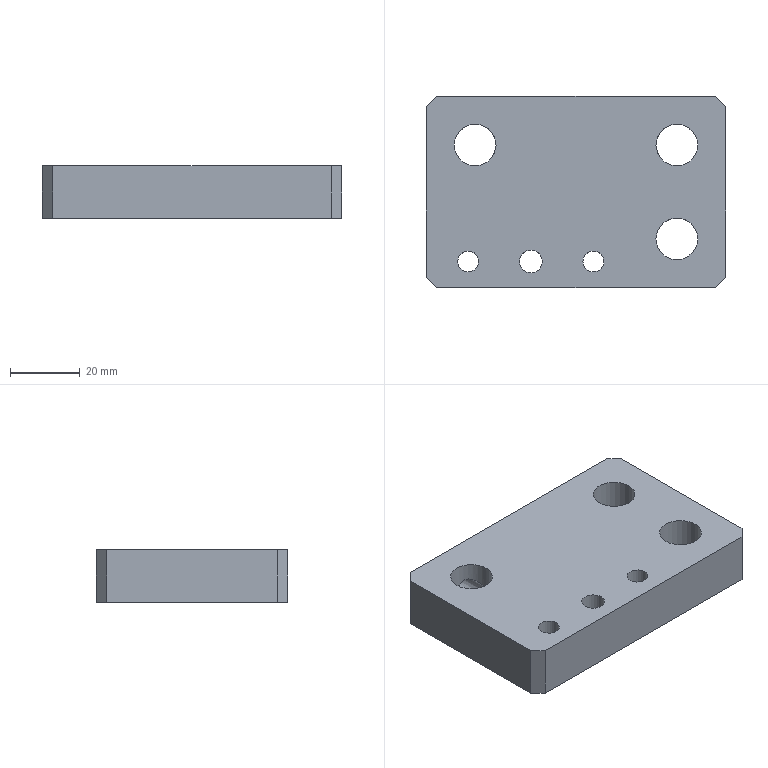Part | NX | features BREP 1 | 1 solid | 26 faces | box 86 x 55 x 15 mm | volume 63166 mm3 | cylinder 12 | plane 11 | cone 3 | commonest cylinder face diameters 5 x5 12 x3 6 x2 6.6 x1 11 x1
STEP:
#1=CARTESIAN_POINT('',(43.,0.,5.));
#2=VERTEX_POINT('',#1);
#3=CARTESIAN_POINT('',(43.,0.,7.5));
#4=DIRECTION('',(1.,0.,0.));
#5=DIRECTION('',(0.,0.,-1.));
#6=AXIS2_PLACEMENT_3D('',#3,#4,#5);
#7=CIRCLE('',#6,2.5);
#8=EDGE_CURVE('',#2,#2,#7,.T.);
#9=ORIENTED_EDGE('',*,*,#8,.F.);
#10=EDGE_LOOP('',(#9));
#11=FACE_BOUND('',#10,.T.);
#12=CARTESIAN_POINT('',(43.,-24.5,15.));
#13=VERTEX_POINT('',#12);
#14=CARTESIAN_POINT('',(43.,24.5,15.));
#15=VERTEX_POINT('',#14);
#16=CARTESIAN_POINT('',(43.,27.5,15.));
#17=DIRECTION('',(0.,1.,0.));
#18=VECTOR('',#17,1000.);
#19=LINE('',#16,#18);
#20=EDGE_CURVE('',#13,#15,#19,.T.);
#21=ORIENTED_EDGE('',*,*,#20,.F.);
#22=CARTESIAN_POINT('',(43.,-24.5,0.));
#23=VERTEX_POINT('',#22);
#24=CARTESIAN_POINT('',(43.,-24.5,15.));
#25=DIRECTION('',(0.,0.,-1.));
#26=VECTOR('',#25,1000.);
#27=LINE('',#24,#26);
#28=EDGE_CURVE('',#13,#23,#27,.T.);
#29=ORIENTED_EDGE('',*,*,#28,.T.);
#30=CARTESIAN_POINT('',(43.,24.5,0.));
#31=VERTEX_POINT('',#30);
#32=CARTESIAN_POINT('',(43.,27.5,0.));
#33=DIRECTION('',(0.,1.,0.));
#34=VECTOR('',#33,1000.);
#35=LINE('',#32,#34);
#36=EDGE_CURVE('',#23,#31,#35,.T.);
#37=ORIENTED_EDGE('',*,*,#36,.T.);
#38=CARTESIAN_POINT('',(43.,24.5,15.));
#39=DIRECTION('',(0.,0.,1.));
#40=VECTOR('',#39,1000.);
#41=LINE('',#38,#40);
#42=EDGE_CURVE('',#31,#15,#41,.T.);
#43=ORIENTED_EDGE('',*,*,#42,.T.);
#44=EDGE_LOOP('',(#21,#29,#37,#43));
#45=FACE_BOUND('',#44,.T.);
#46=CARTESIAN_POINT('',(43.,27.5,15.));
#47=DIRECTION('',(-1.,0.,0.));
#48=DIRECTION('',(0.,1.,0.));
#49=AXIS2_PLACEMENT_3D('',#46,#47,#48);
#50=PLANE('',#49);
#51=ADVANCED_FACE('',(#11,#45),#50,.F.);
#52=CARTESIAN_POINT('',(25.5,27.5,10.));
#53=VERTEX_POINT('',#52);
#54=CARTESIAN_POINT('',(25.5,27.5,7.5));
#55=DIRECTION('',(0.,1.,0.));
#56=DIRECTION('',(0.,0.,1.));
#57=AXIS2_PLACEMENT_3D('',#54,#55,#56);
#58=CIRCLE('',#57,2.5);
#59=EDGE_CURVE('',#53,#53,#58,.T.);
#60=ORIENTED_EDGE('',*,*,#59,.F.);
#61=EDGE_LOOP('',(#60));
#62=FACE_BOUND('',#61,.T.);
#63=CARTESIAN_POINT('',(-25.5,27.5,10.));
#64=VERTEX_POINT('',#63);
#65=CARTESIAN_POINT('',(-25.5,27.5,7.5));
#66=DIRECTION('',(0.,1.,0.));
#67=DIRECTION('',(0.,0.,1.));
#68=AXIS2_PLACEMENT_3D('',#65,#66,#67);
#69=CIRCLE('',#68,2.5);
#70=EDGE_CURVE('',#64,#64,#69,.T.);
#71=ORIENTED_EDGE('',*,*,#70,.F.);
#72=EDGE_LOOP('',(#71));
#73=FACE_BOUND('',#72,.T.);
#74=CARTESIAN_POINT('',(40.,27.5,0.));
#75=VERTEX_POINT('',#74);
#76=CARTESIAN_POINT('',(-40.,27.5,0.));
#77=VERTEX_POINT('',#76);
#78=CARTESIAN_POINT('',(-43.,27.5,0.));
#79=DIRECTION('',(-1.,0.,0.));
#80=VECTOR('',#79,1000.);
#81=LINE('',#78,#80);
#82=EDGE_CURVE('',#75,#77,#81,.T.);
#83=ORIENTED_EDGE('',*,*,#82,.T.);
#84=CARTESIAN_POINT('',(-40.,27.5,15.));
#85=VERTEX_POINT('',#84);
#86=CARTESIAN_POINT('',(-40.,27.5,15.));
#87=DIRECTION('',(0.,0.,1.));
#88=VECTOR('',#87,1000.);
#89=LINE('',#86,#88);
#90=EDGE_CURVE('',#77,#85,#89,.T.);
#91=ORIENTED_EDGE('',*,*,#90,.T.);
#92=CARTESIAN_POINT('',(40.,27.5,15.));
#93=VERTEX_POINT('',#92);
#94=CARTESIAN_POINT('',(-43.,27.5,15.));
#95=DIRECTION('',(-1.,0.,0.));
#96=VECTOR('',#95,1000.);
#97=LINE('',#94,#96);
#98=EDGE_CURVE('',#93,#85,#97,.T.);
#99=ORIENTED_EDGE('',*,*,#98,.F.);
#100=CARTESIAN_POINT('',(40.,27.5,15.));
#101=DIRECTION('',(0.,0.,-1.));
#102=VECTOR('',#101,1000.);
#103=LINE('',#100,#102);
#104=EDGE_CURVE('',#93,#75,#103,.T.);
#105=ORIENTED_EDGE('',*,*,#104,.T.);
#106=EDGE_LOOP('',(#83,#91,#99,#105));
#107=FACE_BOUND('',#106,.T.);
#108=CARTESIAN_POINT('',(-43.,27.5,15.));
#109=DIRECTION('',(0.,-1.,0.));
#110=DIRECTION('',(0.,0.,1.));
#111=AXIS2_PLACEMENT_3D('',#108,#109,#110);
#112=PLANE('',#111);
#113=ADVANCED_FACE('',(#62,#73,#107),#112,.F.);
#114=CARTESIAN_POINT('',(-43.,24.5,0.));
#115=VERTEX_POINT('',#114);
#116=CARTESIAN_POINT('',(-43.,-24.5,0.));
#117=VERTEX_POINT('',#116);
#118=CARTESIAN_POINT('',(-43.,27.5,0.));
#119=DIRECTION('',(0.,-1.,0.));
#120=VECTOR('',#119,1000.);
#121=LINE('',#118,#120);
#122=EDGE_CURVE('',#115,#117,#121,.T.);
#123=ORIENTED_EDGE('',*,*,#122,.T.);
#124=CARTESIAN_POINT('',(-43.,-24.5,15.));
#125=VERTEX_POINT('',#124);
#126=CARTESIAN_POINT('',(-43.,-24.5,15.));
#127=DIRECTION('',(0.,0.,1.));
#128=VECTOR('',#127,1000.);
#129=LINE('',#126,#128);
#130=EDGE_CURVE('',#117,#125,#129,.T.);
#131=ORIENTED_EDGE('',*,*,#130,.T.);
#132=CARTESIAN_POINT('',(-43.,24.5,15.));
#133=VERTEX_POINT('',#132);
#134=CARTESIAN_POINT('',(-43.,27.5,15.));
#135=DIRECTION('',(0.,-1.,0.));
#136=VECTOR('',#135,1000.);
#137=LINE('',#134,#136);
#138=EDGE_CURVE('',#133,#125,#137,.T.);
#139=ORIENTED_EDGE('',*,*,#138,.F.);
#140=CARTESIAN_POINT('',(-43.,24.5,15.));
#141=DIRECTION('',(0.,0.,-1.));
#142=VECTOR('',#141,1000.);
#143=LINE('',#140,#142);
#144=EDGE_CURVE('',#133,#115,#143,.T.);
#145=ORIENTED_EDGE('',*,*,#144,.T.);
#146=EDGE_LOOP('',(#123,#131,#139,#145));
#147=FACE_BOUND('',#146,.T.);
#148=CARTESIAN_POINT('',(-43.,27.5,15.));
#149=DIRECTION('',(1.,0.,0.));
#150=DIRECTION('',(0.,-1.,0.));
#151=AXIS2_PLACEMENT_3D('',#148,#149,#150);
#152=PLANE('',#151);
#153=ADVANCED_FACE('',(#147),#152,.F.);
#154=CARTESIAN_POINT('',(-40.,-27.5,15.));
#155=VERTEX_POINT('',#154);
#156=CARTESIAN_POINT('',(40.,-27.5,15.));
#157=VERTEX_POINT('',#156);
#158=CARTESIAN_POINT('',(-43.,-27.5,15.));
#159=DIRECTION('',(1.,0.,0.));
#160=VECTOR('',#159,1000.);
#161=LINE('',#158,#160);
#162=EDGE_CURVE('',#155,#157,#161,.T.);
#163=ORIENTED_EDGE('',*,*,#162,.F.);
#164=CARTESIAN_POINT('',(-40.,-27.5,0.));
#165=VERTEX_POINT('',#164);
#166=CARTESIAN_POINT('',(-40.,-27.5,15.));
#167=DIRECTION('',(0.,0.,-1.));
#168=VECTOR('',#167,1000.);
#169=LINE('',#166,#168);
#170=EDGE_CURVE('',#155,#165,#169,.T.);
#171=ORIENTED_EDGE('',*,*,#170,.T.);
#172=CARTESIAN_POINT('',(40.,-27.5,0.));
#173=VERTEX_POINT('',#172);
#174=CARTESIAN_POINT('',(-43.,-27.5,0.));
#175=DIRECTION('',(1.,0.,0.));
#176=VECTOR('',#175,1000.);
#177=LINE('',#174,#176);
#178=EDGE_CURVE('',#165,#173,#177,.T.);
#179=ORIENTED_EDGE('',*,*,#178,.T.);
#180=CARTESIAN_POINT('',(40.,-27.5,15.));
#181=DIRECTION('',(0.,0.,1.));
#182=VECTOR('',#181,1000.);
#183=LINE('',#180,#182);
#184=EDGE_CURVE('',#173,#157,#183,.T.);
#185=ORIENTED_EDGE('',*,*,#184,.T.);
#186=EDGE_LOOP('',(#163,#171,#179,#185));
#187=FACE_BOUND('',#186,.T.);
#188=CARTESIAN_POINT('',(-43.,-27.5,15.));
#189=DIRECTION('',(0.,1.,0.));
#190=DIRECTION('',(0.,0.,-1.));
#191=AXIS2_PLACEMENT_3D('',#188,#189,#190);
#192=PLANE('',#191);
#193=ADVANCED_FACE('',(#187),#192,.F.);
#194=CARTESIAN_POINT('',(-16.3,-20.,15.));
#195=VERTEX_POINT('',#194);
#196=CARTESIAN_POINT('',(-13.,-20.,15.));
#197=DIRECTION('',(0.,0.,-1.));
#198=DIRECTION('',(-1.,0.,0.));
#199=AXIS2_PLACEMENT_3D('',#196,#197,#198);
#200=CIRCLE('',#199,3.3);
#201=EDGE_CURVE('',#195,#195,#200,.T.);
#202=ORIENTED_EDGE('',*,*,#201,.T.);
#203=EDGE_LOOP('',(#202));
#204=FACE_BOUND('',#203,.T.);
#205=CARTESIAN_POINT('',(8.,-20.,15.));
#206=VERTEX_POINT('',#205);
#207=CARTESIAN_POINT('',(5.,-20.,15.));
#208=DIRECTION('',(0.,0.,1.));
#209=DIRECTION('',(1.,0.,0.));
#210=AXIS2_PLACEMENT_3D('',#207,#208,#209);
#211=CIRCLE('',#210,3.);
#212=EDGE_CURVE('',#206,#206,#211,.T.);
#213=ORIENTED_EDGE('',*,*,#212,.F.);
#214=EDGE_LOOP('',(#213));
#215=FACE_BOUND('',#214,.T.);
#216=CARTESIAN_POINT('',(-28.,-20.,15.));
#217=VERTEX_POINT('',#216);
#218=CARTESIAN_POINT('',(-31.,-20.,15.));
#219=DIRECTION('',(0.,0.,1.));
#220=DIRECTION('',(1.,0.,0.));
#221=AXIS2_PLACEMENT_3D('',#218,#219,#220);
#222=CIRCLE('',#221,3.);
#223=EDGE_CURVE('',#217,#217,#222,.T.);
#224=ORIENTED_EDGE('',*,*,#223,.F.);
#225=EDGE_LOOP('',(#224));
#226=FACE_BOUND('',#225,.T.);
#227=CARTESIAN_POINT('',(-23.,13.5,15.));
#228=VERTEX_POINT('',#227);
#229=CARTESIAN_POINT('',(-29.,13.5,15.));
#230=DIRECTION('',(0.,0.,1.));
#231=DIRECTION('',(1.,0.,0.));
#232=AXIS2_PLACEMENT_3D('',#229,#230,#231);
#233=CIRCLE('',#232,6.);
#234=EDGE_CURVE('',#228,#228,#233,.T.);
#235=ORIENTED_EDGE('',*,*,#234,.F.);
#236=EDGE_LOOP('',(#235));
#237=FACE_BOUND('',#236,.T.);
#238=CARTESIAN_POINT('',(35.,13.5,15.));
#239=VERTEX_POINT('',#238);
#240=CARTESIAN_POINT('',(29.,13.5,15.));
#241=DIRECTION('',(0.,0.,1.));
#242=DIRECTION('',(1.,0.,0.));
#243=AXIS2_PLACEMENT_3D('',#240,#241,#242);
#244=CIRCLE('',#243,6.);
#245=EDGE_CURVE('',#239,#239,#244,.T.);
#246=ORIENTED_EDGE('',*,*,#245,.F.);
#247=EDGE_LOOP('',(#246));
#248=FACE_BOUND('',#247,.T.);
#249=CARTESIAN_POINT('',(35.,-13.5,15.));
#250=VERTEX_POINT('',#249);
#251=CARTESIAN_POINT('',(29.,-13.5,15.));
#252=DIRECTION('',(0.,0.,1.));
#253=DIRECTION('',(1.,0.,0.));
#254=AXIS2_PLACEMENT_3D('',#251,#252,#253);
#255=CIRCLE('',#254,6.);
#256=EDGE_CURVE('',#250,#250,#255,.T.);
#257=ORIENTED_EDGE('',*,*,#256,.F.);
#258=EDGE_LOOP('',(#257));
#259=FACE_BOUND('',#258,.T.);
#260=ORIENTED_EDGE('',*,*,#138,.T.);
#261=CARTESIAN_POINT('',(-33.75,-33.75,15.));
#262=DIRECTION('',(0.7071,-0.7071,0.));
#263=VECTOR('',#262,1000.);
#264=LINE('',#261,#263);
#265=EDGE_CURVE('',#125,#155,#264,.T.);
#266=ORIENTED_EDGE('',*,*,#265,.T.);
#267=ORIENTED_EDGE('',*,*,#162,.T.);
#268=CARTESIAN_POINT('',(33.75,-33.75,15.));
#269=DIRECTION('',(0.7071,0.7071,0.));
#270=VECTOR('',#269,1000.);
#271=LINE('',#268,#270);
#272=EDGE_CURVE('',#157,#13,#271,.T.);
#273=ORIENTED_EDGE('',*,*,#272,.T.);
#274=ORIENTED_EDGE('',*,*,#20,.T.);
#275=CARTESIAN_POINT('',(33.75,33.75,15.));
#276=DIRECTION('',(-0.7071,0.7071,0.));
#277=VECTOR('',#276,1000.);
#278=LINE('',#275,#277);
#279=EDGE_CURVE('',#15,#93,#278,.T.);
#280=ORIENTED_EDGE('',*,*,#279,.T.);
#281=ORIENTED_EDGE('',*,*,#98,.T.);
#282=CARTESIAN_POINT('',(-33.75,33.75,15.));
#283=DIRECTION('',(-0.7071,-0.7071,0.));
#284=VECTOR('',#283,1000.);
#285=LINE('',#282,#284);
#286=EDGE_CURVE('',#85,#133,#285,.T.);
#287=ORIENTED_EDGE('',*,*,#286,.T.);
#288=EDGE_LOOP('',(#260,#266,#267,#273,#274,#280,#281,#287));
#289=FACE_BOUND('',#288,.T.);
#290=CARTESIAN_POINT('',(0.,0.,15.));
#291=DIRECTION('',(0.,0.,1.));
#292=DIRECTION('',(-1.,0.,0.));
#293=AXIS2_PLACEMENT_3D('',#290,#291,#292);
#294=PLANE('',#293);
#295=ADVANCED_FACE('',(#204,#215,#226,#237,#248,#259,#289),#294,.T.);
#296=CARTESIAN_POINT('',(-18.5,-20.,0.));
#297=VERTEX_POINT('',#296);
#298=CARTESIAN_POINT('',(-13.,-20.,0.));
#299=DIRECTION('',(0.,0.,-1.));
#300=DIRECTION('',(-1.,0.,0.));
#301=AXIS2_PLACEMENT_3D('',#298,#299,#300);
#302=CIRCLE('',#301,5.5);
#303=EDGE_CURVE('',#297,#297,#302,.T.);
#304=ORIENTED_EDGE('',*,*,#303,.F.);
#305=EDGE_LOOP('',(#304));
#306=FACE_BOUND('',#305,.T.);
#307=CARTESIAN_POINT('',(8.,-20.,0.));
#308=VERTEX_POINT('',#307);
#309=CARTESIAN_POINT('',(5.,-20.,0.));
#310=DIRECTION('',(0.,0.,1.));
#311=DIRECTION('',(1.,0.,0.));
#312=AXIS2_PLACEMENT_3D('',#309,#310,#311);
#313=CIRCLE('',#312,3.);
#314=EDGE_CURVE('',#308,#308,#313,.T.);
#315=ORIENTED_EDGE('',*,*,#314,.T.);
#316=EDGE_LOOP('',(#315));
#317=FACE_BOUND('',#316,.T.);
#318=CARTESIAN_POINT('',(-28.,-20.,0.));
#319=VERTEX_POINT('',#318);
#320=CARTESIAN_POINT('',(-31.,-20.,0.));
#321=DIRECTION('',(0.,0.,1.));
#322=DIRECTION('',(1.,0.,0.));
#323=AXIS2_PLACEMENT_3D('',#320,#321,#322);
#324=CIRCLE('',#323,3.);
#325=EDGE_CURVE('',#319,#319,#324,.T.);
#326=ORIENTED_EDGE('',*,*,#325,.T.);
#327=EDGE_LOOP('',(#326));
#328=FACE_BOUND('',#327,.T.);
#329=CARTESIAN_POINT('',(-23.,13.5,0.));
#330=VERTEX_POINT('',#329);
#331=CARTESIAN_POINT('',(-29.,13.5,0.));
#332=DIRECTION('',(0.,0.,1.));
#333=DIRECTION('',(1.,0.,0.));
#334=AXIS2_PLACEMENT_3D('',#331,#332,#333);
#335=CIRCLE('',#334,6.);
#336=EDGE_CURVE('',#330,#330,#335,.T.);
#337=ORIENTED_EDGE('',*,*,#336,.T.);
#338=EDGE_LOOP('',(#337));
#339=FACE_BOUND('',#338,.T.);
#340=CARTESIAN_POINT('',(35.,13.5,0.));
#341=VERTEX_POINT('',#340);
#342=CARTESIAN_POINT('',(29.,13.5,0.));
#343=DIRECTION('',(0.,0.,1.));
#344=DIRECTION('',(1.,0.,0.));
#345=AXIS2_PLACEMENT_3D('',#342,#343,#344);
#346=CIRCLE('',#345,6.);
#347=EDGE_CURVE('',#341,#341,#346,.T.);
#348=ORIENTED_EDGE('',*,*,#347,.T.);
#349=EDGE_LOOP('',(#348));
#350=FACE_BOUND('',#349,.T.);
#351=CARTESIAN_POINT('',(35.,-13.5,0.));
#352=VERTEX_POINT('',#351);
#353=CARTESIAN_POINT('',(29.,-13.5,0.));
#354=DIRECTION('',(0.,0.,1.));
#355=DIRECTION('',(1.,0.,0.));
#356=AXIS2_PLACEMENT_3D('',#353,#354,#355);
#357=CIRCLE('',#356,6.);
#358=EDGE_CURVE('',#352,#352,#357,.T.);
#359=ORIENTED_EDGE('',*,*,#358,.T.);
#360=EDGE_LOOP('',(#359));
#361=FACE_BOUND('',#360,.T.);
#362=ORIENTED_EDGE('',*,*,#178,.F.);
#363=CARTESIAN_POINT('',(-40.,-27.5,0.));
#364=DIRECTION('',(-0.7071,0.7071,0.));
#365=VECTOR('',#364,1000.);
#366=LINE('',#363,#365);
#367=EDGE_CURVE('',#165,#117,#366,.T.);
#368=ORIENTED_EDGE('',*,*,#367,.T.);
#369=ORIENTED_EDGE('',*,*,#122,.F.);
#370=CARTESIAN_POINT('',(-43.,24.5,0.));
#371=DIRECTION('',(0.7071,0.7071,0.));
#372=VECTOR('',#371,1000.);
#373=LINE('',#370,#372);
#374=EDGE_CURVE('',#115,#77,#373,.T.);
#375=ORIENTED_EDGE('',*,*,#374,.T.);
#376=ORIENTED_EDGE('',*,*,#82,.F.);
#377=CARTESIAN_POINT('',(40.,27.5,0.));
#378=DIRECTION('',(0.7071,-0.7071,0.));
#379=VECTOR('',#378,1000.);
#380=LINE('',#377,#379);
#381=EDGE_CURVE('',#75,#31,#380,.T.);
#382=ORIENTED_EDGE('',*,*,#381,.T.);
#383=ORIENTED_EDGE('',*,*,#36,.F.);
#384=CARTESIAN_POINT('',(43.,-24.5,0.));
#385=DIRECTION('',(-0.7071,-0.7071,0.));
#386=VECTOR('',#385,1000.);
#387=LINE('',#384,#386);
#388=EDGE_CURVE('',#23,#173,#387,.T.);
#389=ORIENTED_EDGE('',*,*,#388,.T.);
#390=EDGE_LOOP('',(#362,#368,#369,#375,#376,#382,#383,#389));
#391=FACE_BOUND('',#390,.T.);
#392=CARTESIAN_POINT('',(0.,0.,0.));
#393=DIRECTION('',(0.,0.,1.));
#394=DIRECTION('',(-1.,0.,0.));
#395=AXIS2_PLACEMENT_3D('',#392,#393,#394);
#396=PLANE('',#395);
#397=ADVANCED_FACE('',(#306,#317,#328,#339,#350,#361,#391),#396,.F.);
#398=ORIENTED_EDGE('',*,*,#358,.F.);
#399=EDGE_LOOP('',(#398));
#400=FACE_BOUND('',#399,.T.);
#401=ORIENTED_EDGE('',*,*,#256,.T.);
#402=EDGE_LOOP('',(#401));
#403=FACE_BOUND('',#402,.T.);
#404=CARTESIAN_POINT('',(29.,-13.5,15.));
#405=DIRECTION('',(0.,0.,1.));
#406=DIRECTION('',(-1.,0.,0.));
#407=AXIS2_PLACEMENT_3D('',#404,#405,#406);
#408=CYLINDRICAL_SURFACE('',#407,6.);
#409=ADVANCED_FACE('',(#400,#403),#408,.F.);
#410=CARTESIAN_POINT('',(23.084,12.5,6.858));
#411=VERTEX_POINT('',#410);
#412=CARTESIAN_POINT('',(23.084,12.5,8.142));
#413=VERTEX_POINT('',#412);
#414=CARTESIAN_POINT('',(23.084,12.5,6.858));
#415=CARTESIAN_POINT('',(23.096,12.427,7.286));
#416=CARTESIAN_POINT('',(23.096,12.427,7.714));
#417=CARTESIAN_POINT('',(23.084,12.5,8.142));
#418=B_SPLINE_CURVE_WITH_KNOTS('',3,(#414,#415,#416,#417),.UNSPECIFIED.,.F.,.F.,(4,4),(0.,0.001285),.UNSPECIFIED.);
#419=EDGE_CURVE('',#411,#413,#418,.T.);
#420=ORIENTED_EDGE('',*,*,#419,.T.);
#421=CARTESIAN_POINT('',(23.,13.5,7.5));
#422=VERTEX_POINT('',#421);
#423=CARTESIAN_POINT('',(23.084,12.5,8.142));
#424=CARTESIAN_POINT('',(23.028,12.833,7.931));
#425=CARTESIAN_POINT('',(23.,13.166,7.715));
#426=CARTESIAN_POINT('',(23.,13.5,7.5));
#427=B_SPLINE_CURVE_WITH_KNOTS('',3,(#423,#424,#425,#426),.UNSPECIFIED.,.F.,.F.,(4,4),(0.,0.001192),.UNSPECIFIED.);
#428=EDGE_CURVE('',#413,#422,#427,.T.);
#429=ORIENTED_EDGE('',*,*,#428,.T.);
#430=CARTESIAN_POINT('',(23.,13.5,7.5));
#431=CARTESIAN_POINT('',(23.,13.489,7.507));
#432=CARTESIAN_POINT('',(23.,13.554,7.529));
#433=CARTESIAN_POINT('',(23.001,13.593,7.564));
#434=CARTESIAN_POINT('',(23.003,13.701,7.627));
#435=CARTESIAN_POINT('',(23.008,13.826,7.711));
#436=CARTESIAN_POINT('',(23.018,13.975,7.806));
#437=CARTESIAN_POINT('',(23.035,14.156,7.922));
#438=CARTESIAN_POINT('',(23.062,14.364,8.056));
#439=CARTESIAN_POINT('',(23.098,14.598,8.205));
#440=CARTESIAN_POINT('',(23.219,15.142,8.546));
#441=CARTESIAN_POINT('',(23.366,15.588,8.819));
#442=CARTESIAN_POINT('',(23.62,16.178,9.163));
#443=CARTESIAN_POINT('',(23.871,16.632,9.411));
#444=CARTESIAN_POINT('',(24.252,17.186,9.68));
#445=CARTESIAN_POINT('',(24.615,17.611,9.853));
#446=CARTESIAN_POINT('',(25.124,18.096,9.989));
#447=CARTESIAN_POINT('',(25.768,18.585,10.026));
#448=CARTESIAN_POINT('',(26.575,19.014,9.827));
#449=CARTESIAN_POINT('',(27.257,19.248,9.318));
#450=CARTESIAN_POINT('',(27.671,19.354,8.797));
#451=CARTESIAN_POINT('',(27.932,19.405,8.192));
#452=CARTESIAN_POINT('',(28.029,19.421,7.538));
#453=CARTESIAN_POINT('',(27.952,19.408,6.882));
#454=CARTESIAN_POINT('',(27.71,19.363,6.272));
#455=CARTESIAN_POINT('',(27.32,19.266,5.747));
#456=CARTESIAN_POINT('',(26.664,19.05,5.219));
#457=CARTESIAN_POINT('',(25.881,18.654,4.989));
#458=CARTESIAN_POINT('',(25.232,18.185,4.997));
#459=CARTESIAN_POINT('',(24.71,17.71,5.113));
#460=CARTESIAN_POINT('',(24.336,17.291,5.273));
#461=CARTESIAN_POINT('',(23.941,16.745,5.531));
#462=CARTESIAN_POINT('',(23.679,16.293,5.772));
#463=CARTESIAN_POINT('',(23.41,15.706,6.11));
#464=CARTESIAN_POINT('',(23.252,15.247,6.388));
#465=CARTESIAN_POINT('',(23.098,14.635,6.77));
#466=CARTESIAN_POINT('',(23.033,14.179,7.063));
#467=CARTESIAN_POINT('',(23.008,13.839,7.281));
#468=CARTESIAN_POINT('',(23.002,13.67,7.391));
#469=CARTESIAN_POINT('',(23.001,13.584,7.446));
#470=CARTESIAN_POINT('',(23.,13.542,7.473));
#471=CARTESIAN_POINT('',(23.,13.521,7.486));
#472=CARTESIAN_POINT('',(23.,13.511,7.493));
#473=CARTESIAN_POINT('',(23.,13.505,7.497));
#474=CARTESIAN_POINT('',(23.,13.503,7.498));
#475=CARTESIAN_POINT('',(23.,13.501,7.499));
#476=CARTESIAN_POINT('',(23.,13.501,7.5));
#477=CARTESIAN_POINT('',(23.,13.5,7.5));
#478=CARTESIAN_POINT('',(23.,13.489,7.507));
#479=CARTESIAN_POINT('',(23.,13.554,7.529));
#480=B_SPLINE_CURVE_WITH_KNOTS('',3,(#430,#431,#432,#433,#434,#435,#436,#437,#438,#439,#440,#441,#442,#443,#444,#445,#446,#447,#448,#449,#450,#451,#452,#453,#454,#455,#456,#457,#458,#459,#460,#461,#462,#463,#464,#465,#466,#467,#468,#469,#470,#471,#472,#473,#474,#475,#476,#477,#478,#479),.UNSPECIFIED.,.T.,.F.,(1,1,1,1,1,1,1,1,1,1,1,1,1,1,1,1,1,1,1,1,1,1,1,1,1,1,1,1,1,1,1,1,1,1,1,1,1,1,1,1,1,1,1,1,1,1,1,1,1,1,1,1,1,1),(-0.00006443,-0.00003221,-0.00001611,0.,0.001855,0.003711,0.007422,0.01484,0.02227,0.02969,0.04453,0.05937,0.09055,0.1217,0.153,0.1842,0.2155,0.2467,0.278,0.3092,0.3717,0.4045,0.4359,0.4671,0.4984,0.5296,0.5609,0.5921,0.6234,0.6843,0.7155,0.7467,0.778,0.8092,0.8405,0.8717,0.903,0.9342,0.967,0.9835,0.9918,0.9959,0.9979,0.999,0.9995,0.9997,0.9999,0.9999,1.,1.,1.,1.002,1.004,1.007),.UNSPECIFIED.);
#481=EDGE_CURVE('',#422,#422,#480,.T.);
#482=ORIENTED_EDGE('',*,*,#481,.T.);
#483=CARTESIAN_POINT('',(23.,13.5,7.5));
#484=CARTESIAN_POINT('',(23.,13.167,7.285));
#485=CARTESIAN_POINT('',(23.028,12.831,7.068));
#486=CARTESIAN_POINT('',(23.084,12.5,6.858));
#487=B_SPLINE_CURVE_WITH_KNOTS('',3,(#483,#484,#485,#486),.UNSPECIFIED.,.F.,.F.,(4,4),(-0.00001549,0.001172),.UNSPECIFIED.);
#488=EDGE_CURVE('',#422,#411,#487,.T.);
#489=ORIENTED_EDGE('',*,*,#488,.T.);
#490=EDGE_LOOP('',(#420,#429,#482,#489));
#491=FACE_BOUND('',#490,.T.);
#492=ORIENTED_EDGE('',*,*,#347,.F.);
#493=EDGE_LOOP('',(#492));
#494=FACE_BOUND('',#493,.T.);
#495=ORIENTED_EDGE('',*,*,#245,.T.);
#496=EDGE_LOOP('',(#495));
#497=FACE_BOUND('',#496,.T.);
#498=CARTESIAN_POINT('',(29.,13.5,15.));
#499=DIRECTION('',(0.,0.,1.));
#500=DIRECTION('',(-1.,0.,0.));
#501=AXIS2_PLACEMENT_3D('',#498,#499,#500);
#502=CYLINDRICAL_SURFACE('',#501,6.);
#503=ADVANCED_FACE('',(#491,#494,#497),#502,.F.);
#504=CARTESIAN_POINT('',(-23.084,12.5,8.142));
#505=VERTEX_POINT('',#504);
#506=CARTESIAN_POINT('',(-23.084,12.5,6.858));
#507=VERTEX_POINT('',#506);
#508=CARTESIAN_POINT('',(-23.084,12.5,8.142));
#509=CARTESIAN_POINT('',(-23.096,12.427,7.714));
#510=CARTESIAN_POINT('',(-23.096,12.427,7.286));
#511=CARTESIAN_POINT('',(-23.084,12.5,6.858));
#512=B_SPLINE_CURVE_WITH_KNOTS('',3,(#508,#509,#510,#511),.UNSPECIFIED.,.F.,.F.,(4,4),(0.,0.001285),.UNSPECIFIED.);
#513=EDGE_CURVE('',#505,#507,#512,.T.);
#514=ORIENTED_EDGE('',*,*,#513,.T.);
#515=CARTESIAN_POINT('',(-23.,13.5,7.5));
#516=VERTEX_POINT('',#515);
#517=CARTESIAN_POINT('',(-23.084,12.5,6.858));
#518=CARTESIAN_POINT('',(-23.028,12.833,7.069));
#519=CARTESIAN_POINT('',(-23.,13.166,7.285));
#520=CARTESIAN_POINT('',(-23.,13.5,7.5));
#521=B_SPLINE_CURVE_WITH_KNOTS('',3,(#517,#518,#519,#520),.UNSPECIFIED.,.F.,.F.,(4,4),(0.,0.001192),.UNSPECIFIED.);
#522=EDGE_CURVE('',#507,#516,#521,.T.);
#523=ORIENTED_EDGE('',*,*,#522,.T.);
#524=CARTESIAN_POINT('',(-23.,13.5,7.5));
#525=CARTESIAN_POINT('',(-23.,13.489,7.493));
#526=CARTESIAN_POINT('',(-23.,13.554,7.471));
#527=CARTESIAN_POINT('',(-23.001,13.593,7.436));
#528=CARTESIAN_POINT('',(-23.003,13.701,7.373));
#529=CARTESIAN_POINT('',(-23.008,13.826,7.289));
#530=CARTESIAN_POINT('',(-23.018,13.975,7.194));
#531=CARTESIAN_POINT('',(-23.035,14.156,7.078));
#532=CARTESIAN_POINT('',(-23.062,14.364,6.944));
#533=CARTESIAN_POINT('',(-23.098,14.598,6.795));
#534=CARTESIAN_POINT('',(-23.219,15.142,6.454));
#535=CARTESIAN_POINT('',(-23.366,15.588,6.181));
#536=CARTESIAN_POINT('',(-23.62,16.178,5.837));
#537=CARTESIAN_POINT('',(-23.871,16.632,5.589));
#538=CARTESIAN_POINT('',(-24.252,17.186,5.32));
#539=CARTESIAN_POINT('',(-24.615,17.611,5.147));
#540=CARTESIAN_POINT('',(-25.124,18.096,5.011));
#541=CARTESIAN_POINT('',(-25.768,18.585,4.974));
#542=CARTESIAN_POINT('',(-26.575,19.014,5.173));
#543=CARTESIAN_POINT('',(-27.257,19.248,5.682));
#544=CARTESIAN_POINT('',(-27.671,19.354,6.203));
#545=CARTESIAN_POINT('',(-27.932,19.405,6.808));
#546=CARTESIAN_POINT('',(-28.029,19.421,7.462));
#547=CARTESIAN_POINT('',(-27.952,19.408,8.118));
#548=CARTESIAN_POINT('',(-27.71,19.363,8.728));
#549=CARTESIAN_POINT('',(-27.32,19.266,9.253));
#550=CARTESIAN_POINT('',(-26.664,19.05,9.781));
#551=CARTESIAN_POINT('',(-25.881,18.654,10.011));
#552=CARTESIAN_POINT('',(-25.232,18.185,10.003));
#553=CARTESIAN_POINT('',(-24.71,17.71,9.887));
#554=CARTESIAN_POINT('',(-24.336,17.291,9.727));
#555=CARTESIAN_POINT('',(-23.941,16.745,9.469));
#556=CARTESIAN_POINT('',(-23.679,16.293,9.228));
#557=CARTESIAN_POINT('',(-23.41,15.706,8.89));
#558=CARTESIAN_POINT('',(-23.252,15.247,8.612));
#559=CARTESIAN_POINT('',(-23.098,14.635,8.23));
#560=CARTESIAN_POINT('',(-23.033,14.179,7.937));
#561=CARTESIAN_POINT('',(-23.008,13.839,7.719));
#562=CARTESIAN_POINT('',(-23.002,13.67,7.609));
#563=CARTESIAN_POINT('',(-23.001,13.584,7.554));
#564=CARTESIAN_POINT('',(-23.,13.542,7.527));
#565=CARTESIAN_POINT('',(-23.,13.521,7.514));
#566=CARTESIAN_POINT('',(-23.,13.511,7.507));
#567=CARTESIAN_POINT('',(-23.,13.505,7.503));
#568=CARTESIAN_POINT('',(-23.,13.503,7.502));
#569=CARTESIAN_POINT('',(-23.,13.501,7.501));
#570=CARTESIAN_POINT('',(-23.,13.501,7.5));
#571=CARTESIAN_POINT('',(-23.,13.5,7.5));
#572=CARTESIAN_POINT('',(-23.,13.489,7.493));
#573=CARTESIAN_POINT('',(-23.,13.554,7.471));
#574=B_SPLINE_CURVE_WITH_KNOTS('',3,(#524,#525,#526,#527,#528,#529,#530,#531,#532,#533,#534,#535,#536,#537,#538,#539,#540,#541,#542,#543,#544,#545,#546,#547,#548,#549,#550,#551,#552,#553,#554,#555,#556,#557,#558,#559,#560,#561,#562,#563,#564,#565,#566,#567,#568,#569,#570,#571,#572,#573),.UNSPECIFIED.,.T.,.F.,(1,1,1,1,1,1,1,1,1,1,1,1,1,1,1,1,1,1,1,1,1,1,1,1,1,1,1,1,1,1,1,1,1,1,1,1,1,1,1,1,1,1,1,1,1,1,1,1,1,1,1,1,1,1),(-0.00006443,-0.00003221,-0.00001611,0.,0.001855,0.003711,0.007422,0.01484,0.02227,0.02969,0.04453,0.05937,0.09055,0.1217,0.153,0.1842,0.2155,0.2467,0.278,0.3092,0.3717,0.4045,0.4359,0.4671,0.4984,0.5296,0.5609,0.5921,0.6234,0.6843,0.7155,0.7467,0.778,0.8092,0.8405,0.8717,0.903,0.9342,0.967,0.9835,0.9918,0.9959,0.9979,0.999,0.9995,0.9997,0.9999,0.9999,1.,1.,1.,1.002,1.004,1.007),.UNSPECIFIED.);
#575=EDGE_CURVE('',#516,#516,#574,.T.);
#576=ORIENTED_EDGE('',*,*,#575,.T.);
#577=CARTESIAN_POINT('',(-23.084,12.5,8.142));
#578=CARTESIAN_POINT('',(-23.028,12.833,7.931));
#579=CARTESIAN_POINT('',(-23.,13.166,7.715));
#580=CARTESIAN_POINT('',(-23.,13.5,7.5));
#581=B_SPLINE_CURVE_WITH_KNOTS('',3,(#577,#578,#579,#580),.UNSPECIFIED.,.F.,.F.,(4,4),(0.,0.001192),.UNSPECIFIED.);
#582=EDGE_CURVE('',#516,#505,#581,.F.);
#583=ORIENTED_EDGE('',*,*,#582,.T.);
#584=EDGE_LOOP('',(#514,#523,#576,#583));
#585=FACE_BOUND('',#584,.T.);
#586=ORIENTED_EDGE('',*,*,#336,.F.);
#587=EDGE_LOOP('',(#586));
#588=FACE_BOUND('',#587,.T.);
#589=ORIENTED_EDGE('',*,*,#234,.T.);
#590=EDGE_LOOP('',(#589));
#591=FACE_BOUND('',#590,.T.);
#592=CARTESIAN_POINT('',(-29.,13.5,15.));
#593=DIRECTION('',(0.,0.,1.));
#594=DIRECTION('',(-1.,0.,0.));
#595=AXIS2_PLACEMENT_3D('',#592,#593,#594);
#596=CYLINDRICAL_SURFACE('',#595,6.);
#597=ADVANCED_FACE('',(#585,#588,#591),#596,.F.);
#598=ORIENTED_EDGE('',*,*,#265,.F.);
#599=ORIENTED_EDGE('',*,*,#130,.F.);
#600=ORIENTED_EDGE('',*,*,#367,.F.);
#601=ORIENTED_EDGE('',*,*,#170,.F.);
#602=EDGE_LOOP('',(#598,#599,#600,#601));
#603=FACE_BOUND('',#602,.T.);
#604=CARTESIAN_POINT('',(-40.,-27.5,15.));
#605=DIRECTION('',(0.7071,0.7071,0.));
#606=DIRECTION('',(0.,0.,1.));
#607=AXIS2_PLACEMENT_3D('',#604,#605,#606);
#608=PLANE('',#607);
#609=ADVANCED_FACE('',(#603),#608,.F.);
#610=ORIENTED_EDGE('',*,*,#286,.F.);
#611=ORIENTED_EDGE('',*,*,#90,.F.);
#612=ORIENTED_EDGE('',*,*,#374,.F.);
#613=ORIENTED_EDGE('',*,*,#144,.F.);
#614=EDGE_LOOP('',(#610,#611,#612,#613));
#615=FACE_BOUND('',#614,.T.);
#616=CARTESIAN_POINT('',(-43.,24.5,15.));
#617=DIRECTION('',(0.7071,-0.7071,0.));
#618=DIRECTION('',(0.,0.,1.));
#619=AXIS2_PLACEMENT_3D('',#616,#617,#618);
#620=PLANE('',#619);
#621=ADVANCED_FACE('',(#615),#620,.F.);
#622=ORIENTED_EDGE('',*,*,#272,.F.);
#623=ORIENTED_EDGE('',*,*,#184,.F.);
#624=ORIENTED_EDGE('',*,*,#388,.F.);
#625=ORIENTED_EDGE('',*,*,#28,.F.);
#626=EDGE_LOOP('',(#622,#623,#624,#625));
#627=FACE_BOUND('',#626,.T.);
#628=CARTESIAN_POINT('',(43.,-24.5,15.));
#629=DIRECTION('',(-0.7071,0.7071,0.));
#630=DIRECTION('',(0.,0.,1.));
#631=AXIS2_PLACEMENT_3D('',#628,#629,#630);
#632=PLANE('',#631);
#633=ADVANCED_FACE('',(#627),#632,.F.);
#634=ORIENTED_EDGE('',*,*,#279,.F.);
#635=ORIENTED_EDGE('',*,*,#42,.F.);
#636=ORIENTED_EDGE('',*,*,#381,.F.);
#637=ORIENTED_EDGE('',*,*,#104,.F.);
#638=EDGE_LOOP('',(#634,#635,#636,#637));
#639=FACE_BOUND('',#638,.T.);
#640=CARTESIAN_POINT('',(40.,27.5,15.));
#641=DIRECTION('',(-0.7071,-0.7071,0.));
#642=DIRECTION('',(0.,0.,1.));
#643=AXIS2_PLACEMENT_3D('',#640,#641,#642);
#644=PLANE('',#643);
#645=ADVANCED_FACE('',(#639),#644,.F.);
#646=ORIENTED_EDGE('',*,*,#325,.F.);
#647=EDGE_LOOP('',(#646));
#648=FACE_BOUND('',#647,.T.);
#649=ORIENTED_EDGE('',*,*,#223,.T.);
#650=EDGE_LOOP('',(#649));
#651=FACE_BOUND('',#650,.T.);
#652=CARTESIAN_POINT('',(-31.,-20.,15.));
#653=DIRECTION('',(0.,0.,1.));
#654=DIRECTION('',(-1.,0.,0.));
#655=AXIS2_PLACEMENT_3D('',#652,#653,#654);
#656=CYLINDRICAL_SURFACE('',#655,3.);
#657=ADVANCED_FACE('',(#648,#651),#656,.F.);
#658=ORIENTED_EDGE('',*,*,#314,.F.);
#659=EDGE_LOOP('',(#658));
#660=FACE_BOUND('',#659,.T.);
#661=ORIENTED_EDGE('',*,*,#212,.T.);
#662=EDGE_LOOP('',(#661));
#663=FACE_BOUND('',#662,.T.);
#664=CARTESIAN_POINT('',(5.,-20.,15.));
#665=DIRECTION('',(0.,0.,1.));
#666=DIRECTION('',(-1.,0.,0.));
#667=AXIS2_PLACEMENT_3D('',#664,#665,#666);
#668=CYLINDRICAL_SURFACE('',#667,3.);
#669=ADVANCED_FACE('',(#660,#663),#668,.F.);
#670=ORIENTED_EDGE('',*,*,#201,.F.);
#671=EDGE_LOOP('',(#670));
#672=FACE_BOUND('',#671,.T.);
#673=CARTESIAN_POINT('',(-16.3,-20.,6.4));
#674=VERTEX_POINT('',#673);
#675=CARTESIAN_POINT('',(-13.,-20.,6.4));
#676=DIRECTION('',(0.,0.,-1.));
#677=DIRECTION('',(-1.,0.,0.));
#678=AXIS2_PLACEMENT_3D('',#675,#676,#677);
#679=CIRCLE('',#678,3.3);
#680=EDGE_CURVE('',#674,#674,#679,.T.);
#681=ORIENTED_EDGE('',*,*,#680,.T.);
#682=EDGE_LOOP('',(#681));
#683=FACE_BOUND('',#682,.T.);
#684=CARTESIAN_POINT('',(-13.,-20.,0.));
#685=DIRECTION('',(0.,0.,-1.));
#686=DIRECTION('',(1.,0.,0.));
#687=AXIS2_PLACEMENT_3D('',#684,#685,#686);
#688=CYLINDRICAL_SURFACE('',#687,3.3);
#689=ADVANCED_FACE('',(#672,#683),#688,.F.);
#690=ORIENTED_EDGE('',*,*,#680,.F.);
#691=EDGE_LOOP('',(#690));
#692=FACE_BOUND('',#691,.T.);
#693=CARTESIAN_POINT('',(-18.5,-20.,6.4));
#694=VERTEX_POINT('',#693);
#695=CARTESIAN_POINT('',(-13.,-20.,6.4));
#696=DIRECTION('',(0.,0.,-1.));
#697=DIRECTION('',(-1.,0.,0.));
#698=AXIS2_PLACEMENT_3D('',#695,#696,#697);
#699=CIRCLE('',#698,5.5);
#700=EDGE_CURVE('',#694,#694,#699,.T.);
#701=ORIENTED_EDGE('',*,*,#700,.T.);
#702=EDGE_LOOP('',(#701));
#703=FACE_BOUND('',#702,.T.);
#704=CARTESIAN_POINT('',(-9.7,-20.,6.4));
#705=DIRECTION('',(0.,0.,1.));
#706=DIRECTION('',(-1.,0.,0.));
#707=AXIS2_PLACEMENT_3D('',#704,#705,#706);
#708=PLANE('',#707);
#709=ADVANCED_FACE('',(#692,#703),#708,.F.);
#710=ORIENTED_EDGE('',*,*,#700,.F.);
#711=EDGE_LOOP('',(#710));
#712=FACE_BOUND('',#711,.T.);
#713=ORIENTED_EDGE('',*,*,#303,.T.);
#714=EDGE_LOOP('',(#713));
#715=FACE_BOUND('',#714,.T.);
#716=CARTESIAN_POINT('',(-13.,-20.,0.));
#717=DIRECTION('',(0.,0.,-1.));
#718=DIRECTION('',(1.,0.,0.));
#719=AXIS2_PLACEMENT_3D('',#716,#717,#718);
#720=CYLINDRICAL_SURFACE('',#719,5.5);
#721=ADVANCED_FACE('',(#712,#715),#720,.F.);
#722=CARTESIAN_POINT('',(26.498,0.,7.5));
#723=VERTEX_POINT('',#722);
#724=VERTEX_LOOP('',#723);
#725=FACE_BOUND('',#724,.T.);
#726=CARTESIAN_POINT('',(28.,0.,5.));
#727=VERTEX_POINT('',#726);
#728=CARTESIAN_POINT('',(28.,0.,7.5));
#729=DIRECTION('',(1.,0.,0.));
#730=DIRECTION('',(0.,0.,-1.));
#731=AXIS2_PLACEMENT_3D('',#728,#729,#730);
#732=CIRCLE('',#731,2.5);
#733=EDGE_CURVE('',#727,#727,#732,.T.);
#734=ORIENTED_EDGE('',*,*,#733,.T.);
#735=EDGE_LOOP('',(#734));
#736=FACE_BOUND('',#735,.T.);
#737=CARTESIAN_POINT('',(28.,0.,7.5));
#738=DIRECTION('',(1.,0.,0.));
#739=DIRECTION('',(0.,0.,1.));
#740=AXIS2_PLACEMENT_3D('',#737,#738,#739);
#741=CONICAL_SURFACE('',#740,2.5,1.03);
#742=ADVANCED_FACE('',(#725,#736),#741,.F.);
#743=ORIENTED_EDGE('',*,*,#733,.F.);
#744=EDGE_LOOP('',(#743));
#745=FACE_BOUND('',#744,.T.);
#746=ORIENTED_EDGE('',*,*,#8,.T.);
#747=EDGE_LOOP('',(#746));
#748=FACE_BOUND('',#747,.T.);
#749=CARTESIAN_POINT('',(43.,0.,7.5));
#750=DIRECTION('',(1.,0.,0.));
#751=DIRECTION('',(0.,0.,1.));
#752=AXIS2_PLACEMENT_3D('',#749,#750,#751);
#753=CYLINDRICAL_SURFACE('',#752,2.5);
#754=ADVANCED_FACE('',(#745,#748),#753,.F.);
#755=ORIENTED_EDGE('',*,*,#70,.T.);
#756=EDGE_LOOP('',(#755));
#757=FACE_BOUND('',#756,.T.);
#758=ORIENTED_EDGE('',*,*,#575,.F.);
#759=EDGE_LOOP('',(#758));
#760=FACE_BOUND('',#759,.T.);
#761=CARTESIAN_POINT('',(-25.5,27.5,7.5));
#762=DIRECTION('',(0.,1.,0.));
#763=DIRECTION('',(0.,0.,-1.));
#764=AXIS2_PLACEMENT_3D('',#761,#762,#763);
#765=CYLINDRICAL_SURFACE('',#764,2.5);
#766=ADVANCED_FACE('',(#757,#760),#765,.F.);
#767=CARTESIAN_POINT('',(-25.5,12.5,7.5));
#768=DIRECTION('',(0.,1.,0.));
#769=DIRECTION('',(0.,0.,1.));
#770=AXIS2_PLACEMENT_3D('',#767,#768,#769);
#771=CIRCLE('',#770,2.5);
#772=EDGE_CURVE('',#505,#507,#771,.T.);
#773=ORIENTED_EDGE('',*,*,#772,.T.);
#774=ORIENTED_EDGE('',*,*,#513,.F.);
#775=EDGE_LOOP('',(#773,#774));
#776=FACE_BOUND('',#775,.T.);
#777=CARTESIAN_POINT('',(-25.5,12.5,7.5));
#778=DIRECTION('',(0.,1.,0.));
#779=DIRECTION('',(0.,0.,-1.));
#780=AXIS2_PLACEMENT_3D('',#777,#778,#779);
#781=CONICAL_SURFACE('',#780,2.5,1.03);
#782=ADVANCED_FACE('',(#776),#781,.F.);
#783=ORIENTED_EDGE('',*,*,#772,.F.);
#784=ORIENTED_EDGE('',*,*,#582,.F.);
#785=ORIENTED_EDGE('',*,*,#522,.F.);
#786=EDGE_LOOP('',(#783,#784,#785));
#787=FACE_BOUND('',#786,.T.);
#788=CARTESIAN_POINT('',(-25.5,27.5,7.5));
#789=DIRECTION('',(0.,1.,0.));
#790=DIRECTION('',(0.,0.,-1.));
#791=AXIS2_PLACEMENT_3D('',#788,#789,#790);
#792=CYLINDRICAL_SURFACE('',#791,2.5);
#793=ADVANCED_FACE('',(#787),#792,.F.);
#794=ORIENTED_EDGE('',*,*,#59,.T.);
#795=EDGE_LOOP('',(#794));
#796=FACE_BOUND('',#795,.T.);
#797=ORIENTED_EDGE('',*,*,#481,.F.);
#798=EDGE_LOOP('',(#797));
#799=FACE_BOUND('',#798,.T.);
#800=CARTESIAN_POINT('',(25.5,27.5,7.5));
#801=DIRECTION('',(0.,1.,0.));
#802=DIRECTION('',(0.,0.,-1.));
#803=AXIS2_PLACEMENT_3D('',#800,#801,#802);
#804=CYLINDRICAL_SURFACE('',#803,2.5);
#805=ADVANCED_FACE('',(#796,#799),#804,.F.);
#806=CARTESIAN_POINT('',(25.5,12.5,7.5));
#807=DIRECTION('',(0.,1.,0.));
#808=DIRECTION('',(0.,0.,1.));
#809=AXIS2_PLACEMENT_3D('',#806,#807,#808);
#810=CIRCLE('',#809,2.5);
#811=EDGE_CURVE('',#411,#413,#810,.T.);
#812=ORIENTED_EDGE('',*,*,#811,.T.);
#813=ORIENTED_EDGE('',*,*,#419,.F.);
#814=EDGE_LOOP('',(#812,#813));
#815=FACE_BOUND('',#814,.T.);
#816=CARTESIAN_POINT('',(25.5,12.5,7.5));
#817=DIRECTION('',(0.,1.,0.));
#818=DIRECTION('',(0.,0.,-1.));
#819=AXIS2_PLACEMENT_3D('',#816,#817,#818);
#820=CONICAL_SURFACE('',#819,2.5,1.03);
#821=ADVANCED_FACE('',(#815),#820,.F.);
#822=ORIENTED_EDGE('',*,*,#811,.F.);
#823=ORIENTED_EDGE('',*,*,#488,.F.);
#824=ORIENTED_EDGE('',*,*,#428,.F.);
#825=EDGE_LOOP('',(#822,#823,#824));
#826=FACE_BOUND('',#825,.T.);
#827=CARTESIAN_POINT('',(25.5,27.5,7.5));
#828=DIRECTION('',(0.,1.,0.));
#829=DIRECTION('',(0.,0.,-1.));
#830=AXIS2_PLACEMENT_3D('',#827,#828,#829);
#831=CYLINDRICAL_SURFACE('',#830,2.5);
#832=ADVANCED_FACE('',(#826),#831,.F.);
#833=CLOSED_SHELL('',(#51,#113,#153,#193,#295,#397,#409,#503,#597,#609,#621,#633,#645,#657,#669,#689,#709,#721,#742,#754,#766,#782,#793,#805,#821,#832));
#834=MANIFOLD_SOLID_BREP('',#833);
#835=(LENGTH_UNIT()NAMED_UNIT(*)SI_UNIT(.MILLI.,.METRE.));
#836=UNCERTAINTY_MEASURE_WITH_UNIT(LENGTH_MEASURE(0.0508),#835,'','');
#837=(NAMED_UNIT(*)PLANE_ANGLE_UNIT()SI_UNIT($,.RADIAN.));
#838=(NAMED_UNIT(*)SI_UNIT($,.STERADIAN.)SOLID_ANGLE_UNIT());
#839=(GEOMETRIC_REPRESENTATION_CONTEXT(3)GLOBAL_UNCERTAINTY_ASSIGNED_CONTEXT((#836))GLOBAL_UNIT_ASSIGNED_CONTEXT((#835,#837,#838))REPRESENTATION_CONTEXT('',''));
#840=ADVANCED_BREP_SHAPE_REPRESENTATION('',(#834),#839);